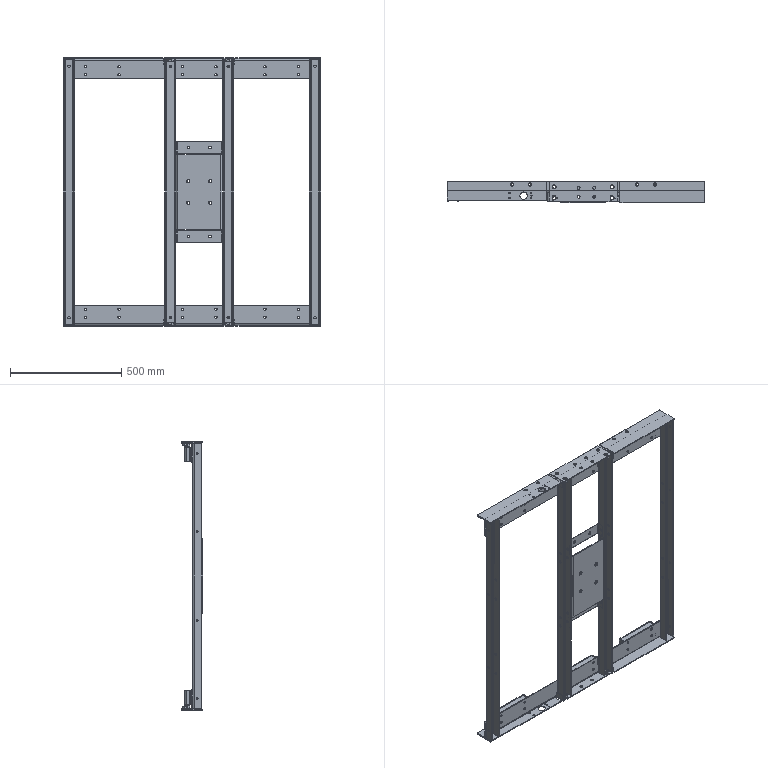Part | SolidWorks | features ReferencePattern 18, MirrorCompFeat 6, CompositeCurve 1 | 53 solids | 1486 faces | box 1155 x 95 x 1206 mm | volume 5315222 mm3 | plane 838 | cylinder 528 | cone 120 | commonest cylinder face diameters 11 x136 16 x56 10.5 x48 13 x48 8 x40 12 x28